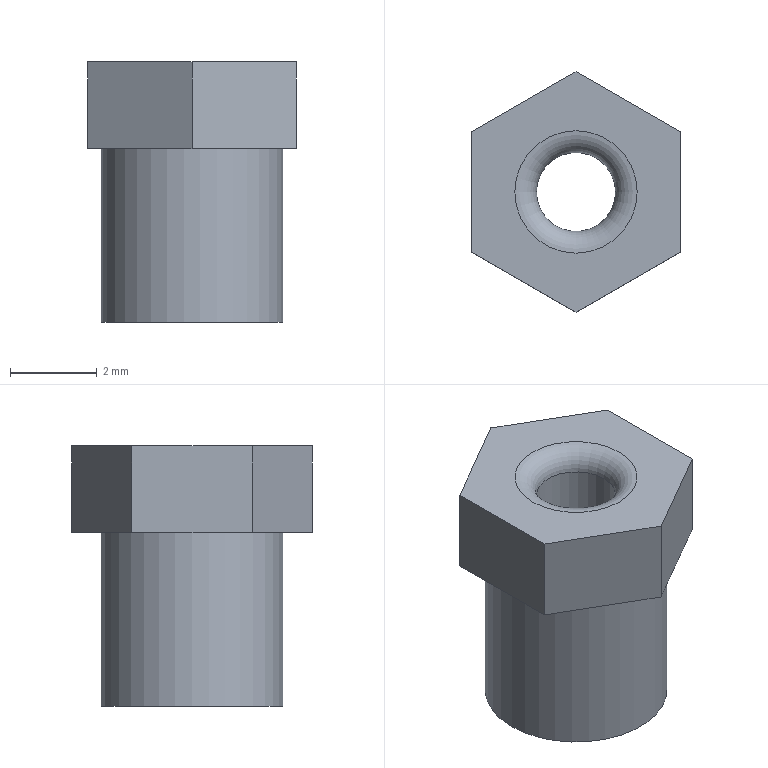Part | NX | features BREP 1 | 1 solid | 14 faces | box 4.8 x 5.543 x 6 mm | volume 57.333 mm3 | plane 10 | cylinder 3 | torus 1 | commonest cylinder face diameters 1.822 x1 3.2 x1 4.19 x1
STEP:
#1=CARTESIAN_POINT('',(-2.058,3.451,-4.));
#2=VERTEX_POINT('',#1);
#3=CARTESIAN_POINT('',(-3.658,3.451,-4.));
#4=DIRECTION('',(0.,0.,1.));
#5=DIRECTION('',(1.,0.,0.));
#6=AXIS2_PLACEMENT_3D('',#3,#4,#5);
#7=CIRCLE('',#6,1.6);
#8=EDGE_CURVE('',#2,#2,#7,.T.);
#9=ORIENTED_EDGE('',*,*,#8,.F.);
#10=EDGE_LOOP('',(#9));
#11=FACE_BOUND('',#10,.T.);
#12=CARTESIAN_POINT('',(-2.058,3.451,0.));
#13=VERTEX_POINT('',#12);
#14=CARTESIAN_POINT('',(-3.658,3.451,0.));
#15=DIRECTION('',(0.,0.,-1.));
#16=DIRECTION('',(1.,0.,0.));
#17=AXIS2_PLACEMENT_3D('',#14,#15,#16);
#18=CIRCLE('',#17,1.6);
#19=EDGE_CURVE('',#13,#13,#18,.T.);
#20=ORIENTED_EDGE('',*,*,#19,.F.);
#21=EDGE_LOOP('',(#20));
#22=FACE_BOUND('',#21,.T.);
#23=CARTESIAN_POINT('',(-3.658,3.451,0.));
#24=DIRECTION('',(0.,0.,-1.));
#25=DIRECTION('',(1.,0.,0.));
#26=AXIS2_PLACEMENT_3D('',#23,#24,#25);
#27=CYLINDRICAL_SURFACE('',#26,1.6);
#28=ADVANCED_FACE('',(#11,#22),#27,.F.);
#29=CARTESIAN_POINT('',(-1.563,3.451,-4.));
#30=VERTEX_POINT('',#29);
#31=CARTESIAN_POINT('',(-3.658,3.451,-4.));
#32=DIRECTION('',(0.,0.,1.));
#33=DIRECTION('',(1.,0.,0.));
#34=AXIS2_PLACEMENT_3D('',#31,#32,#33);
#35=CIRCLE('',#34,2.095);
#36=EDGE_CURVE('',#30,#30,#35,.T.);
#37=ORIENTED_EDGE('',*,*,#36,.T.);
#38=EDGE_LOOP('',(#37));
#39=FACE_BOUND('',#38,.T.);
#40=CARTESIAN_POINT('',(-1.563,3.451,0.));
#41=VERTEX_POINT('',#40);
#42=CARTESIAN_POINT('',(-3.658,3.451,0.));
#43=DIRECTION('',(0.,0.,1.));
#44=DIRECTION('',(1.,0.,0.));
#45=AXIS2_PLACEMENT_3D('',#42,#43,#44);
#46=CIRCLE('',#45,2.095);
#47=EDGE_CURVE('',#41,#41,#46,.T.);
#48=ORIENTED_EDGE('',*,*,#47,.F.);
#49=EDGE_LOOP('',(#48));
#50=FACE_BOUND('',#49,.T.);
#51=CARTESIAN_POINT('',(-3.658,3.451,0.));
#52=DIRECTION('',(0.,0.,-1.));
#53=DIRECTION('',(1.,0.,0.));
#54=AXIS2_PLACEMENT_3D('',#51,#52,#53);
#55=CYLINDRICAL_SURFACE('',#54,2.095);
#56=ADVANCED_FACE('',(#39,#50),#55,.T.);
#57=ORIENTED_EDGE('',*,*,#36,.F.);
#58=EDGE_LOOP('',(#57));
#59=FACE_BOUND('',#58,.T.);
#60=ORIENTED_EDGE('',*,*,#8,.T.);
#61=EDGE_LOOP('',(#60));
#62=FACE_BOUND('',#61,.T.);
#63=CARTESIAN_POINT('',(-3.658,3.451,-4.));
#64=DIRECTION('',(0.,0.,1.));
#65=DIRECTION('',(1.,0.,0.));
#66=AXIS2_PLACEMENT_3D('',#63,#64,#65);
#67=PLANE('',#66);
#68=ADVANCED_FACE('',(#59,#62),#67,.F.);
#69=CARTESIAN_POINT('',(-1.258,4.837,0.));
#70=VERTEX_POINT('',#69);
#71=CARTESIAN_POINT('',(-1.258,2.065,0.));
#72=VERTEX_POINT('',#71);
#73=CARTESIAN_POINT('',(-1.258,4.837,0.));
#74=DIRECTION('',(0.,-1.,0.));
#75=VECTOR('',#74,1000.);
#76=LINE('',#73,#75);
#77=EDGE_CURVE('',#70,#72,#76,.T.);
#78=ORIENTED_EDGE('',*,*,#77,.T.);
#79=CARTESIAN_POINT('',(-3.658,0.6797,0.));
#80=VERTEX_POINT('',#79);
#81=CARTESIAN_POINT('',(-1.258,2.065,0.));
#82=DIRECTION('',(-0.866,-0.5,0.));
#83=VECTOR('',#82,1000.);
#84=LINE('',#81,#83);
#85=EDGE_CURVE('',#72,#80,#84,.T.);
#86=ORIENTED_EDGE('',*,*,#85,.T.);
#87=CARTESIAN_POINT('',(-6.058,2.065,0.));
#88=VERTEX_POINT('',#87);
#89=CARTESIAN_POINT('',(-3.658,0.6797,0.));
#90=DIRECTION('',(-0.866,0.5,0.));
#91=VECTOR('',#90,1000.);
#92=LINE('',#89,#91);
#93=EDGE_CURVE('',#80,#88,#92,.T.);
#94=ORIENTED_EDGE('',*,*,#93,.T.);
#95=CARTESIAN_POINT('',(-6.058,4.837,0.));
#96=VERTEX_POINT('',#95);
#97=CARTESIAN_POINT('',(-6.058,2.065,0.));
#98=DIRECTION('',(0.,1.,0.));
#99=VECTOR('',#98,1000.);
#100=LINE('',#97,#99);
#101=EDGE_CURVE('',#88,#96,#100,.T.);
#102=ORIENTED_EDGE('',*,*,#101,.T.);
#103=CARTESIAN_POINT('',(-3.658,6.222,0.));
#104=VERTEX_POINT('',#103);
#105=CARTESIAN_POINT('',(-6.058,4.837,0.));
#106=DIRECTION('',(0.866,0.5,0.));
#107=VECTOR('',#106,1000.);
#108=LINE('',#105,#107);
#109=EDGE_CURVE('',#96,#104,#108,.T.);
#110=ORIENTED_EDGE('',*,*,#109,.T.);
#111=CARTESIAN_POINT('',(-3.658,6.222,0.));
#112=DIRECTION('',(0.866,-0.5,0.));
#113=VECTOR('',#112,1000.);
#114=LINE('',#111,#113);
#115=EDGE_CURVE('',#104,#70,#114,.T.);
#116=ORIENTED_EDGE('',*,*,#115,.T.);
#117=EDGE_LOOP('',(#78,#86,#94,#102,#110,#116));
#118=FACE_BOUND('',#117,.T.);
#119=ORIENTED_EDGE('',*,*,#47,.T.);
#120=EDGE_LOOP('',(#119));
#121=FACE_BOUND('',#120,.T.);
#122=CARTESIAN_POINT('',(-3.658,3.451,0.));
#123=DIRECTION('',(0.,0.,1.));
#124=DIRECTION('',(1.,0.,0.));
#125=AXIS2_PLACEMENT_3D('',#122,#123,#124);
#126=PLANE('',#125);
#127=ADVANCED_FACE('',(#118,#121),#126,.F.);
#128=CARTESIAN_POINT('',(-4.569,3.451,1.5));
#129=VERTEX_POINT('',#128);
#130=CARTESIAN_POINT('',(-3.658,3.451,1.5));
#131=DIRECTION('',(0.,0.,-1.));
#132=DIRECTION('',(-1.,0.,0.));
#133=AXIS2_PLACEMENT_3D('',#130,#131,#132);
#134=CIRCLE('',#133,0.9109);
#135=EDGE_CURVE('',#129,#129,#134,.T.);
#136=ORIENTED_EDGE('',*,*,#135,.T.);
#137=EDGE_LOOP('',(#136));
#138=FACE_BOUND('',#137,.T.);
#139=CARTESIAN_POINT('',(-5.069,3.451,2.));
#140=VERTEX_POINT('',#139);
#141=CARTESIAN_POINT('',(-3.658,3.451,2.));
#142=DIRECTION('',(0.,0.,1.));
#143=DIRECTION('',(-1.,0.,0.));
#144=AXIS2_PLACEMENT_3D('',#141,#142,#143);
#145=CIRCLE('',#144,1.411);
#146=EDGE_CURVE('',#140,#140,#145,.T.);
#147=ORIENTED_EDGE('',*,*,#146,.T.);
#148=EDGE_LOOP('',(#147));
#149=FACE_BOUND('',#148,.T.);
#150=CARTESIAN_POINT('',(-3.658,3.451,1.5));
#151=DIRECTION('',(0.,0.,-1.));
#152=DIRECTION('',(-1.,0.,0.));
#153=AXIS2_PLACEMENT_3D('',#150,#151,#152);
#154=TOROIDAL_SURFACE('',#153,1.411,0.5);
#155=ADVANCED_FACE('',(#138,#149),#154,.T.);
#156=CARTESIAN_POINT('',(-4.569,3.451,0.));
#157=VERTEX_POINT('',#156);
#158=CARTESIAN_POINT('',(-3.658,3.451,0.));
#159=DIRECTION('',(0.,0.,1.));
#160=DIRECTION('',(-1.,0.,0.));
#161=AXIS2_PLACEMENT_3D('',#158,#159,#160);
#162=CIRCLE('',#161,0.9109);
#163=EDGE_CURVE('',#157,#157,#162,.T.);
#164=ORIENTED_EDGE('',*,*,#163,.F.);
#165=EDGE_LOOP('',(#164));
#166=FACE_BOUND('',#165,.T.);
#167=ORIENTED_EDGE('',*,*,#135,.F.);
#168=EDGE_LOOP('',(#167));
#169=FACE_BOUND('',#168,.T.);
#170=CARTESIAN_POINT('',(-3.658,3.451,2.));
#171=DIRECTION('',(0.,0.,-1.));
#172=DIRECTION('',(-1.,0.,0.));
#173=AXIS2_PLACEMENT_3D('',#170,#171,#172);
#174=CYLINDRICAL_SURFACE('',#173,0.9109);
#175=ADVANCED_FACE('',(#166,#169),#174,.F.);
#176=CARTESIAN_POINT('',(-1.258,2.065,2.));
#177=VERTEX_POINT('',#176);
#178=CARTESIAN_POINT('',(-3.658,0.6797,2.));
#179=VERTEX_POINT('',#178);
#180=CARTESIAN_POINT('',(-1.258,2.065,2.));
#181=DIRECTION('',(-0.866,-0.5,0.));
#182=VECTOR('',#181,1000.);
#183=LINE('',#180,#182);
#184=EDGE_CURVE('',#177,#179,#183,.T.);
#185=ORIENTED_EDGE('',*,*,#184,.F.);
#186=CARTESIAN_POINT('',(-1.258,4.837,2.));
#187=VERTEX_POINT('',#186);
#188=CARTESIAN_POINT('',(-1.258,4.837,2.));
#189=DIRECTION('',(0.,-1.,0.));
#190=VECTOR('',#189,1000.);
#191=LINE('',#188,#190);
#192=EDGE_CURVE('',#187,#177,#191,.T.);
#193=ORIENTED_EDGE('',*,*,#192,.F.);
#194=CARTESIAN_POINT('',(-3.658,6.222,2.));
#195=VERTEX_POINT('',#194);
#196=CARTESIAN_POINT('',(-3.658,6.222,2.));
#197=DIRECTION('',(0.866,-0.5,0.));
#198=VECTOR('',#197,1000.);
#199=LINE('',#196,#198);
#200=EDGE_CURVE('',#195,#187,#199,.T.);
#201=ORIENTED_EDGE('',*,*,#200,.F.);
#202=CARTESIAN_POINT('',(-6.058,4.837,2.));
#203=VERTEX_POINT('',#202);
#204=CARTESIAN_POINT('',(-6.058,4.837,2.));
#205=DIRECTION('',(0.866,0.5,0.));
#206=VECTOR('',#205,1000.);
#207=LINE('',#204,#206);
#208=EDGE_CURVE('',#203,#195,#207,.T.);
#209=ORIENTED_EDGE('',*,*,#208,.F.);
#210=CARTESIAN_POINT('',(-6.058,2.065,2.));
#211=VERTEX_POINT('',#210);
#212=CARTESIAN_POINT('',(-6.058,2.065,2.));
#213=DIRECTION('',(0.,1.,0.));
#214=VECTOR('',#213,1000.);
#215=LINE('',#212,#214);
#216=EDGE_CURVE('',#211,#203,#215,.T.);
#217=ORIENTED_EDGE('',*,*,#216,.F.);
#218=CARTESIAN_POINT('',(-3.658,0.6797,2.));
#219=DIRECTION('',(-0.866,0.5,0.));
#220=VECTOR('',#219,1000.);
#221=LINE('',#218,#220);
#222=EDGE_CURVE('',#179,#211,#221,.T.);
#223=ORIENTED_EDGE('',*,*,#222,.F.);
#224=EDGE_LOOP('',(#185,#193,#201,#209,#217,#223));
#225=FACE_BOUND('',#224,.T.);
#226=ORIENTED_EDGE('',*,*,#146,.F.);
#227=EDGE_LOOP('',(#226));
#228=FACE_BOUND('',#227,.T.);
#229=CARTESIAN_POINT('',(-3.658,3.451,2.));
#230=DIRECTION('',(0.,0.,1.));
#231=DIRECTION('',(1.,0.,0.));
#232=AXIS2_PLACEMENT_3D('',#229,#230,#231);
#233=PLANE('',#232);
#234=ADVANCED_FACE('',(#225,#228),#233,.T.);
#235=ORIENTED_EDGE('',*,*,#184,.T.);
#236=CARTESIAN_POINT('',(-3.658,0.6797,0.));
#237=DIRECTION('',(0.,0.,1.));
#238=VECTOR('',#237,1000.);
#239=LINE('',#236,#238);
#240=EDGE_CURVE('',#80,#179,#239,.T.);
#241=ORIENTED_EDGE('',*,*,#240,.F.);
#242=ORIENTED_EDGE('',*,*,#85,.F.);
#243=CARTESIAN_POINT('',(-1.258,2.065,0.));
#244=DIRECTION('',(0.,0.,1.));
#245=VECTOR('',#244,1000.);
#246=LINE('',#243,#245);
#247=EDGE_CURVE('',#72,#177,#246,.T.);
#248=ORIENTED_EDGE('',*,*,#247,.T.);
#249=EDGE_LOOP('',(#235,#241,#242,#248));
#250=FACE_BOUND('',#249,.T.);
#251=CARTESIAN_POINT('',(-1.258,2.065,0.));
#252=DIRECTION('',(0.5,-0.866,0.));
#253=DIRECTION('',(0.,0.,-1.));
#254=AXIS2_PLACEMENT_3D('',#251,#252,#253);
#255=PLANE('',#254);
#256=ADVANCED_FACE('',(#250),#255,.T.);
#257=ORIENTED_EDGE('',*,*,#222,.T.);
#258=CARTESIAN_POINT('',(-6.058,2.065,0.));
#259=DIRECTION('',(0.,0.,1.));
#260=VECTOR('',#259,1000.);
#261=LINE('',#258,#260);
#262=EDGE_CURVE('',#88,#211,#261,.T.);
#263=ORIENTED_EDGE('',*,*,#262,.F.);
#264=ORIENTED_EDGE('',*,*,#93,.F.);
#265=ORIENTED_EDGE('',*,*,#240,.T.);
#266=EDGE_LOOP('',(#257,#263,#264,#265));
#267=FACE_BOUND('',#266,.T.);
#268=CARTESIAN_POINT('',(-3.658,0.6797,0.));
#269=DIRECTION('',(-0.5,-0.866,0.));
#270=DIRECTION('',(0.,0.,-1.));
#271=AXIS2_PLACEMENT_3D('',#268,#269,#270);
#272=PLANE('',#271);
#273=ADVANCED_FACE('',(#267),#272,.T.);
#274=ORIENTED_EDGE('',*,*,#216,.T.);
#275=CARTESIAN_POINT('',(-6.058,4.837,0.));
#276=DIRECTION('',(0.,0.,1.));
#277=VECTOR('',#276,1000.);
#278=LINE('',#275,#277);
#279=EDGE_CURVE('',#96,#203,#278,.T.);
#280=ORIENTED_EDGE('',*,*,#279,.F.);
#281=ORIENTED_EDGE('',*,*,#101,.F.);
#282=ORIENTED_EDGE('',*,*,#262,.T.);
#283=EDGE_LOOP('',(#274,#280,#281,#282));
#284=FACE_BOUND('',#283,.T.);
#285=CARTESIAN_POINT('',(-6.058,2.065,0.));
#286=DIRECTION('',(-1.,0.,0.));
#287=DIRECTION('',(0.,0.,1.));
#288=AXIS2_PLACEMENT_3D('',#285,#286,#287);
#289=PLANE('',#288);
#290=ADVANCED_FACE('',(#284),#289,.T.);
#291=ORIENTED_EDGE('',*,*,#208,.T.);
#292=CARTESIAN_POINT('',(-3.658,6.222,0.));
#293=DIRECTION('',(0.,0.,1.));
#294=VECTOR('',#293,1000.);
#295=LINE('',#292,#294);
#296=EDGE_CURVE('',#104,#195,#295,.T.);
#297=ORIENTED_EDGE('',*,*,#296,.F.);
#298=ORIENTED_EDGE('',*,*,#109,.F.);
#299=ORIENTED_EDGE('',*,*,#279,.T.);
#300=EDGE_LOOP('',(#291,#297,#298,#299));
#301=FACE_BOUND('',#300,.T.);
#302=CARTESIAN_POINT('',(-6.058,4.837,0.));
#303=DIRECTION('',(-0.5,0.866,0.));
#304=DIRECTION('',(0.,0.,1.));
#305=AXIS2_PLACEMENT_3D('',#302,#303,#304);
#306=PLANE('',#305);
#307=ADVANCED_FACE('',(#301),#306,.T.);
#308=ORIENTED_EDGE('',*,*,#200,.T.);
#309=CARTESIAN_POINT('',(-1.258,4.837,0.));
#310=DIRECTION('',(0.,0.,1.));
#311=VECTOR('',#310,1000.);
#312=LINE('',#309,#311);
#313=EDGE_CURVE('',#70,#187,#312,.T.);
#314=ORIENTED_EDGE('',*,*,#313,.F.);
#315=ORIENTED_EDGE('',*,*,#115,.F.);
#316=ORIENTED_EDGE('',*,*,#296,.T.);
#317=EDGE_LOOP('',(#308,#314,#315,#316));
#318=FACE_BOUND('',#317,.T.);
#319=CARTESIAN_POINT('',(-3.658,6.222,0.));
#320=DIRECTION('',(0.5,0.866,0.));
#321=DIRECTION('',(0.,0.,1.));
#322=AXIS2_PLACEMENT_3D('',#319,#320,#321);
#323=PLANE('',#322);
#324=ADVANCED_FACE('',(#318),#323,.T.);
#325=ORIENTED_EDGE('',*,*,#192,.T.);
#326=ORIENTED_EDGE('',*,*,#247,.F.);
#327=ORIENTED_EDGE('',*,*,#77,.F.);
#328=ORIENTED_EDGE('',*,*,#313,.T.);
#329=EDGE_LOOP('',(#325,#326,#327,#328));
#330=FACE_BOUND('',#329,.T.);
#331=CARTESIAN_POINT('',(-1.258,4.837,0.));
#332=DIRECTION('',(1.,0.,0.));
#333=DIRECTION('',(0.,0.,-1.));
#334=AXIS2_PLACEMENT_3D('',#331,#332,#333);
#335=PLANE('',#334);
#336=ADVANCED_FACE('',(#330),#335,.T.);
#337=ORIENTED_EDGE('',*,*,#19,.T.);
#338=EDGE_LOOP('',(#337));
#339=FACE_BOUND('',#338,.T.);
#340=ORIENTED_EDGE('',*,*,#163,.T.);
#341=EDGE_LOOP('',(#340));
#342=FACE_BOUND('',#341,.T.);
#343=CARTESIAN_POINT('',(-3.658,3.451,0.));
#344=DIRECTION('',(0.,0.,1.));
#345=DIRECTION('',(1.,0.,0.));
#346=AXIS2_PLACEMENT_3D('',#343,#344,#345);
#347=PLANE('',#346);
#348=ADVANCED_FACE('',(#339,#342),#347,.F.);
#349=CLOSED_SHELL('',(#28,#56,#68,#127,#155,#175,#234,#256,#273,#290,#307,#324,#336,#348));
#350=MANIFOLD_SOLID_BREP('',#349);
#351=(LENGTH_UNIT()NAMED_UNIT(*)SI_UNIT(.MILLI.,.METRE.));
#352=UNCERTAINTY_MEASURE_WITH_UNIT(LENGTH_MEASURE(0.00001),#351,'','');
#353=(NAMED_UNIT(*)PLANE_ANGLE_UNIT()SI_UNIT($,.RADIAN.));
#354=(NAMED_UNIT(*)SI_UNIT($,.STERADIAN.)SOLID_ANGLE_UNIT());
#355=(GEOMETRIC_REPRESENTATION_CONTEXT(3)GLOBAL_UNCERTAINTY_ASSIGNED_CONTEXT((#352))GLOBAL_UNIT_ASSIGNED_CONTEXT((#351,#353,#354))REPRESENTATION_CONTEXT('',''));
#356=ADVANCED_BREP_SHAPE_REPRESENTATION('',(#350),#355);